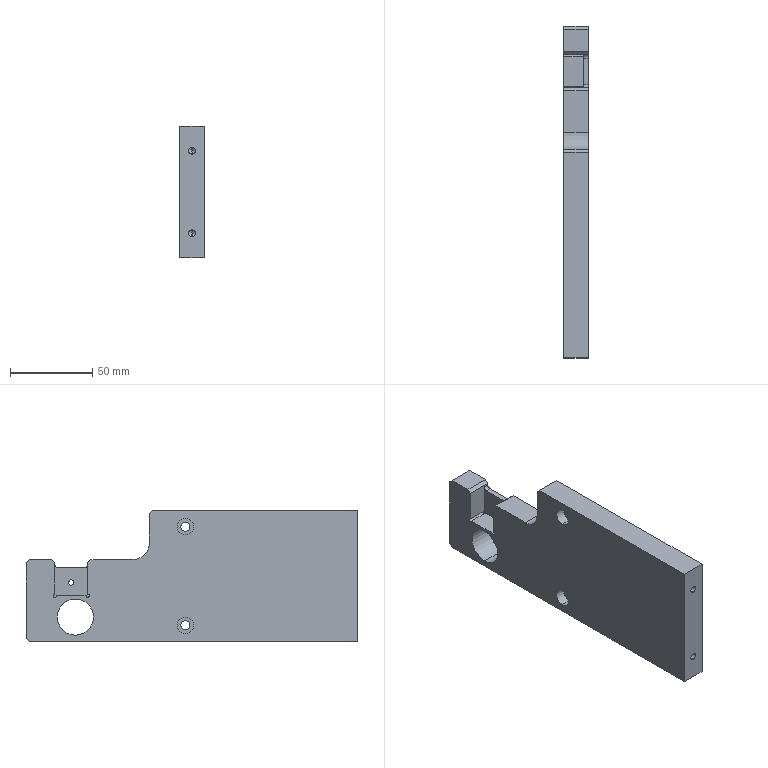Part | SolidWorks | features ICE 6, HoleWzd 4, Chamfer 2, Fillet 2, Cut 1, Extrusion 1 | 1 solid | 54 faces | box 15 x 202 x 80 mm | volume 195162 mm3 | cylinder 25 | plane 21 | cone 8 | commonest cylinder face diameters 4.2 x4 5 x4 5.5 x4 10 x4 2 x2 3.3 x2